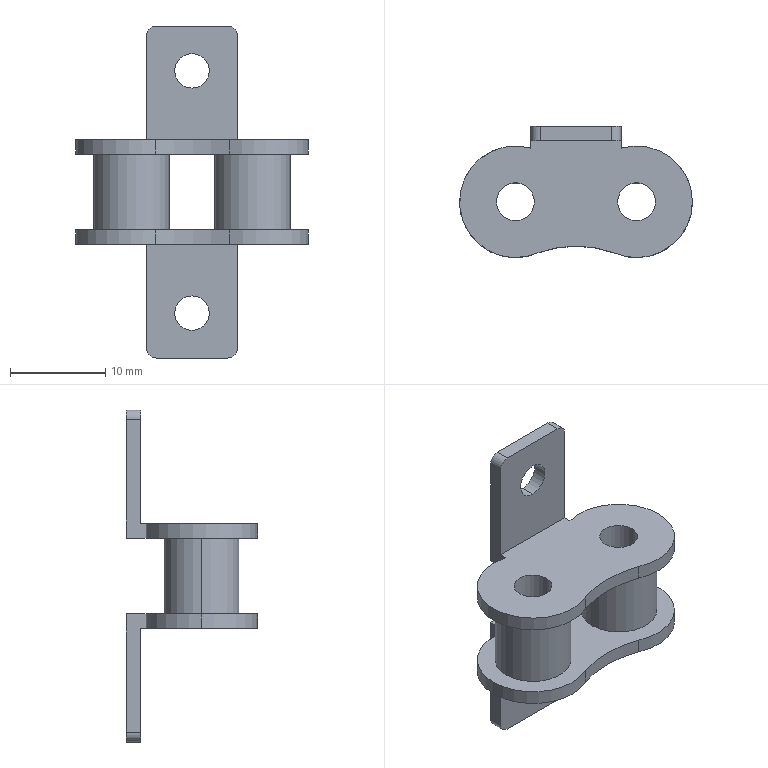Part | STEP file | CHEL40Achain-5 | 1 solid | 38 faces | box 24.4 x 13.75 x 34.8 mm | volume 1627 mm3 | cylinder 24 | plane 14 | commonest cylinder face diameters 11.7 x6 2 x4 3.6 x4 3.97 x4 7.95 x4 23.4 x2